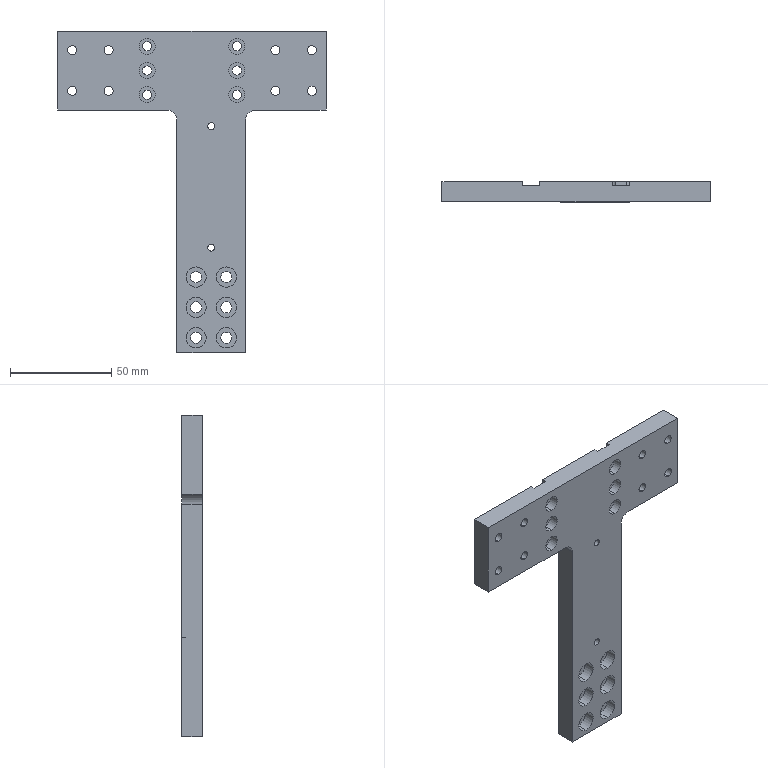Part | STEP file | ASND-0110-TPIM-066 | 1 solid | 134 faces | box 132.4 x 10 x 159 mm | volume 81070 mm3 | cylinder 92 | plane 42 | commonest cylinder face diameters 4.5 x28 8 x28 10 x14 5.5 x12 3 x6 3.4 x4